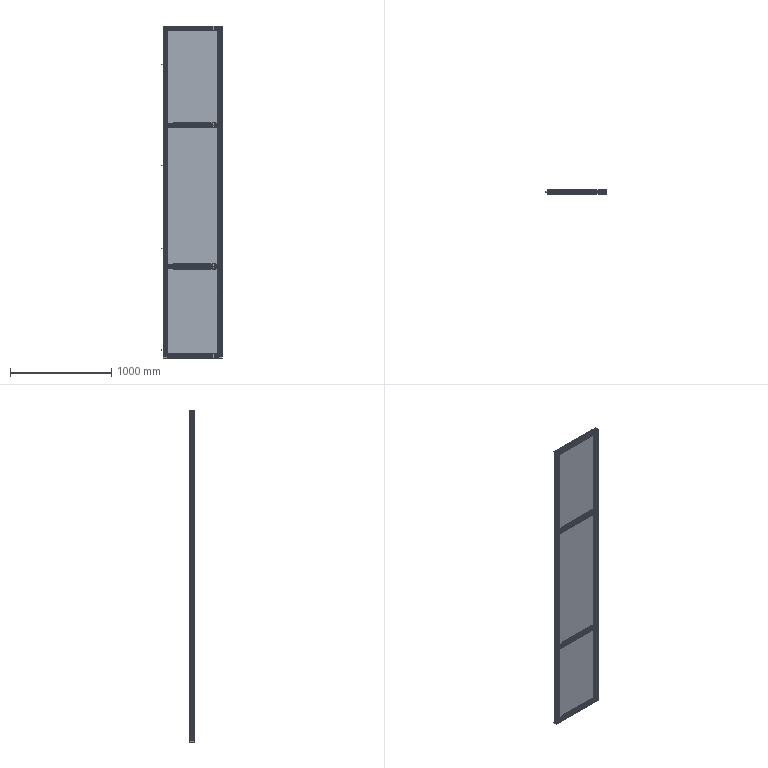Part | SolidWorks | features ReferencePattern 20, LocalLPattern 6 | 45 solids | 2406 faces | box 595.4 x 40 x 3280 mm | volume 13933282 mm3 | plane 1624 | cylinder 714 | cone 60 | spline 8 | commonest cylinder face diameters 6.8 x142 2 x68 19 x48 0.8 x36 1 x36 1.6 x36